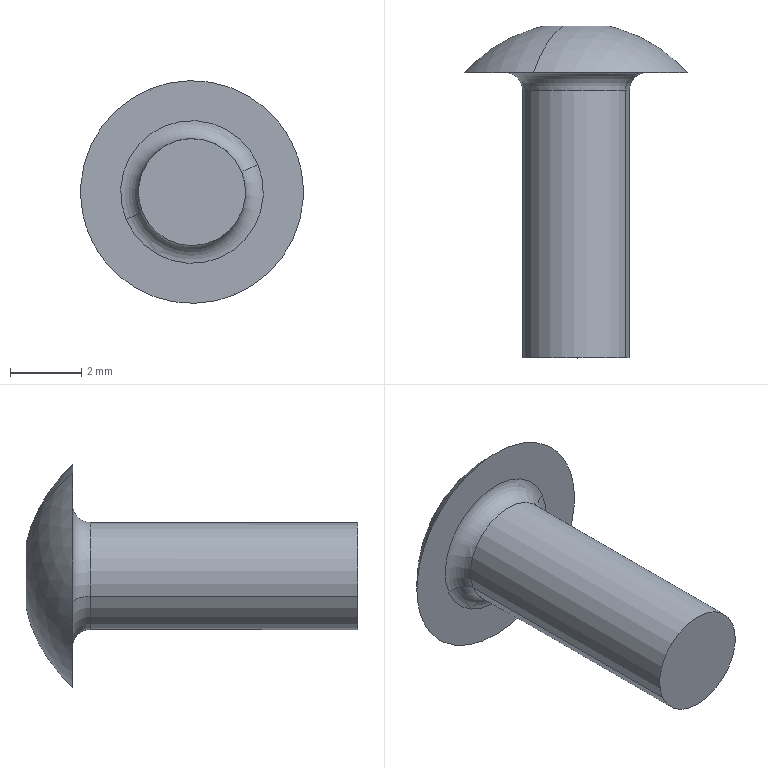Part | SolidWorks | features BaseBody 1 | 1 solid | 9 faces | box 6.24 x 9.303 x 6.24 mm | volume 79.81 mm3 | plane 3 | sphere 2 | torus 2 | cylinder 2 | commonest cylinder face diameters 3 x2
STEP:
#1=CARTESIAN_POINT('',(-240.642,13.167,-31.72));
#2=VERTEX_POINT('',#1);
#3=CARTESIAN_POINT('',(-241.341,14.088,-30.023));
#4=VERTEX_POINT('',#3);
#5=CARTESIAN_POINT('',(-241.684,10.009,-29.193));
#6=DIRECTION('',(0.9245,-0.0001344,0.3811));
#7=DIRECTION('',(0.3811,0.,-0.9245));
#8=AXIS2_PLACEMENT_3D('',#5,#6,#7);
#9=CIRCLE('',#8,4.177);
#10=EDGE_CURVE('',#2,#4,#9,.T.);
#11=ORIENTED_EDGE('',*,*,#10,.F.);
#12=CARTESIAN_POINT('',(-240.495,12.787,-32.076));
#13=VERTEX_POINT('',#12);
#14=CARTESIAN_POINT('',(-241.684,10.009,-29.193));
#15=DIRECTION('',(-0.9245,0.0001344,-0.3811));
#16=DIRECTION('',(-0.3811,0.,0.9245));
#17=AXIS2_PLACEMENT_3D('',#14,#15,#16);
#18=CIRCLE('',#17,4.177);
#19=EDGE_CURVE('',#2,#13,#18,.T.);
#20=ORIENTED_EDGE('',*,*,#19,.T.);
#21=CARTESIAN_POINT('',(-242.873,12.784,-26.307));
#22=VERTEX_POINT('',#21);
#23=CARTESIAN_POINT('',(-241.684,12.786,-29.192));
#24=DIRECTION('',(0.00003827,-1.,-0.0004455));
#25=DIRECTION('',(0.9245,-0.0001344,0.3811));
#26=AXIS2_PLACEMENT_3D('',#23,#24,#25);
#27=CIRCLE('',#26,3.12);
#28=EDGE_CURVE('',#22,#13,#27,.T.);
#29=ORIENTED_EDGE('',*,*,#28,.F.);
#30=CARTESIAN_POINT('',(-242.027,14.087,-28.359));
#31=VERTEX_POINT('',#30);
#32=CARTESIAN_POINT('',(-241.684,10.009,-29.193));
#33=DIRECTION('',(0.9245,-0.0001344,0.3811));
#34=DIRECTION('',(0.3811,0.,-0.9245));
#35=AXIS2_PLACEMENT_3D('',#32,#33,#34);
#36=CIRCLE('',#35,4.177);
#37=EDGE_CURVE('',#31,#22,#36,.T.);
#38=ORIENTED_EDGE('',*,*,#37,.F.);
#39=CARTESIAN_POINT('',(-241.684,14.088,-29.191));
#40=DIRECTION('',(-0.00003827,1.,0.0004455));
#41=DIRECTION('',(0.9245,-0.0001344,0.3811));
#42=AXIS2_PLACEMENT_3D('',#39,#40,#41);
#43=CIRCLE('',#42,0.9);
#44=EDGE_CURVE('',#4,#31,#43,.T.);
#45=ORIENTED_EDGE('',*,*,#44,.F.);
#46=EDGE_LOOP('',(#11,#20,#29,#38,#45));
#47=FACE_OUTER_BOUND('',#46,.T.);
#48=CARTESIAN_POINT('',(-241.684,10.009,-29.193));
#49=DIRECTION('',(-0.9245,0.0001344,-0.3811));
#50=DIRECTION('',(-0.288,0.6545,0.6991));
#51=AXIS2_PLACEMENT_3D('',#48,#49,#50);
#52=SPHERICAL_SURFACE('',#51,4.177);
#53=ADVANCED_FACE('',(#47),#52,.T.);
#54=CARTESIAN_POINT('',(-240.297,12.285,-28.62));
#55=VERTEX_POINT('',#54);
#56=CARTESIAN_POINT('',(-243.071,12.286,-29.763));
#57=VERTEX_POINT('',#56);
#58=CARTESIAN_POINT('',(-241.684,12.286,-29.192));
#59=DIRECTION('',(0.00003827,-1.,-0.0004455));
#60=DIRECTION('',(0.9245,-0.0001344,0.3811));
#61=AXIS2_PLACEMENT_3D('',#58,#59,#60);
#62=CIRCLE('',#61,1.5);
#63=EDGE_CURVE('',#55,#57,#62,.T.);
#64=ORIENTED_EDGE('',*,*,#63,.F.);
#65=CARTESIAN_POINT('',(-239.835,12.785,-28.429));
#66=VERTEX_POINT('',#65);
#67=CARTESIAN_POINT('',(-239.835,12.285,-28.43));
#68=DIRECTION('',(-0.3811,-0.0004264,0.9245));
#69=DIRECTION('',(-0.00003827,1.,0.0004455));
#70=AXIS2_PLACEMENT_3D('',#67,#68,#69);
#71=CIRCLE('',#70,0.5);
#72=EDGE_CURVE('',#66,#55,#71,.T.);
#73=ORIENTED_EDGE('',*,*,#72,.F.);
#74=CARTESIAN_POINT('',(-243.533,12.786,-29.954));
#75=VERTEX_POINT('',#74);
#76=CARTESIAN_POINT('',(-241.684,12.786,-29.192));
#77=DIRECTION('',(0.00003827,-1.,-0.0004455));
#78=DIRECTION('',(0.9245,-0.0001344,0.3811));
#79=AXIS2_PLACEMENT_3D('',#76,#77,#78);
#80=CIRCLE('',#79,2.);
#81=EDGE_CURVE('',#66,#75,#80,.T.);
#82=ORIENTED_EDGE('',*,*,#81,.T.);
#83=CARTESIAN_POINT('',(-243.533,12.286,-29.954));
#84=DIRECTION('',(0.3811,0.0004264,-0.9245));
#85=DIRECTION('',(-0.00003827,1.,0.0004455));
#86=AXIS2_PLACEMENT_3D('',#83,#84,#85);
#87=CIRCLE('',#86,0.5);
#88=EDGE_CURVE('',#75,#57,#87,.T.);
#89=ORIENTED_EDGE('',*,*,#88,.T.);
#90=EDGE_LOOP('',(#64,#73,#82,#89));
#91=FACE_OUTER_BOUND('',#90,.T.);
#92=CARTESIAN_POINT('',(-241.684,12.286,-29.192));
#93=DIRECTION('',(-0.00003827,1.,0.0004455));
#94=DIRECTION('',(-0.9245,0.0001344,-0.3811));
#95=AXIS2_PLACEMENT_3D('',#92,#93,#94);
#96=TOROIDAL_SURFACE('',#95,2.,0.5);
#97=ADVANCED_FACE('',(#91),#96,.F.);
#98=ORIENTED_EDGE('',*,*,#88,.F.);
#99=CARTESIAN_POINT('',(-241.684,12.786,-29.192));
#100=DIRECTION('',(0.00003827,-1.,-0.0004455));
#101=DIRECTION('',(-0.9245,0.0001344,-0.3811));
#102=AXIS2_PLACEMENT_3D('',#99,#100,#101);
#103=CIRCLE('',#102,2.);
#104=EDGE_CURVE('',#75,#66,#103,.T.);
#105=ORIENTED_EDGE('',*,*,#104,.T.);
#106=ORIENTED_EDGE('',*,*,#72,.T.);
#107=CARTESIAN_POINT('',(-241.684,12.286,-29.192));
#108=DIRECTION('',(0.00003827,-1.,-0.0004455));
#109=DIRECTION('',(-0.9245,0.0001344,-0.3811));
#110=AXIS2_PLACEMENT_3D('',#107,#108,#109);
#111=CIRCLE('',#110,1.5);
#112=EDGE_CURVE('',#57,#55,#111,.T.);
#113=ORIENTED_EDGE('',*,*,#112,.F.);
#114=EDGE_LOOP('',(#98,#105,#106,#113));
#115=FACE_OUTER_BOUND('',#114,.T.);
#116=CARTESIAN_POINT('',(-241.684,12.286,-29.192));
#117=DIRECTION('',(-0.00003827,1.,0.0004455));
#118=DIRECTION('',(0.9245,-0.0001344,0.3811));
#119=AXIS2_PLACEMENT_3D('',#116,#117,#118);
#120=TOROIDAL_SURFACE('',#119,2.,0.5);
#121=ADVANCED_FACE('',(#115),#120,.F.);
#122=CARTESIAN_POINT('',(-243.07,4.786,-29.767));
#123=VERTEX_POINT('',#122);
#124=CARTESIAN_POINT('',(-243.071,12.286,-29.763));
#125=DIRECTION('',(0.00003827,-1.,-0.0004455));
#126=VECTOR('',#125,1000.);
#127=LINE('',#124,#126);
#128=EDGE_CURVE('',#57,#123,#127,.T.);
#129=ORIENTED_EDGE('',*,*,#128,.F.);
#130=ORIENTED_EDGE('',*,*,#112,.T.);
#131=CARTESIAN_POINT('',(-240.297,4.785,-28.624));
#132=VERTEX_POINT('',#131);
#133=CARTESIAN_POINT('',(-240.297,12.285,-28.62));
#134=DIRECTION('',(0.00003827,-1.,-0.0004455));
#135=VECTOR('',#134,1000.);
#136=LINE('',#133,#135);
#137=EDGE_CURVE('',#55,#132,#136,.T.);
#138=ORIENTED_EDGE('',*,*,#137,.T.);
#139=CARTESIAN_POINT('',(-241.684,4.786,-29.195));
#140=DIRECTION('',(-0.00003827,1.,0.0004455));
#141=DIRECTION('',(0.9245,-0.0001344,0.3811));
#142=AXIS2_PLACEMENT_3D('',#139,#140,#141);
#143=CIRCLE('',#142,1.5);
#144=EDGE_CURVE('',#132,#123,#143,.T.);
#145=ORIENTED_EDGE('',*,*,#144,.T.);
#146=EDGE_LOOP('',(#129,#130,#138,#145));
#147=FACE_OUTER_BOUND('',#146,.T.);
#148=CARTESIAN_POINT('',(-241.684,24.02,-29.187));
#149=DIRECTION('',(-0.00003827,1.,0.0004455));
#150=DIRECTION('',(0.9245,-0.0001344,0.3811));
#151=AXIS2_PLACEMENT_3D('',#148,#149,#150);
#152=CYLINDRICAL_SURFACE('',#151,1.5);
#153=ADVANCED_FACE('',(#147),#152,.T.);
#154=CARTESIAN_POINT('',(-241.684,4.786,-29.195));
#155=DIRECTION('',(-0.00003827,1.,0.0004455));
#156=DIRECTION('',(-0.9245,0.0001344,-0.3811));
#157=AXIS2_PLACEMENT_3D('',#154,#155,#156);
#158=CIRCLE('',#157,1.5);
#159=EDGE_CURVE('',#123,#132,#158,.T.);
#160=ORIENTED_EDGE('',*,*,#159,.F.);
#161=ORIENTED_EDGE('',*,*,#144,.F.);
#162=EDGE_LOOP('',(#160,#161));
#163=FACE_OUTER_BOUND('',#162,.T.);
#164=CARTESIAN_POINT('',(-242.516,4.786,-29.538));
#165=DIRECTION('',(-0.00003827,1.,0.0004455));
#166=DIRECTION('',(0.9963,0.,0.08559));
#167=AXIS2_PLACEMENT_3D('',#164,#165,#166);
#168=PLANE('',#167);
#169=ADVANCED_FACE('',(#163),#168,.F.);
#170=ORIENTED_EDGE('',*,*,#159,.T.);
#171=ORIENTED_EDGE('',*,*,#137,.F.);
#172=ORIENTED_EDGE('',*,*,#63,.T.);
#173=ORIENTED_EDGE('',*,*,#128,.T.);
#174=EDGE_LOOP('',(#170,#171,#172,#173));
#175=FACE_OUTER_BOUND('',#174,.T.);
#176=CARTESIAN_POINT('',(-241.684,24.02,-29.187));
#177=DIRECTION('',(-0.00003827,1.,0.0004455));
#178=DIRECTION('',(0.9245,-0.0001344,0.3811));
#179=AXIS2_PLACEMENT_3D('',#176,#177,#178);
#180=CYLINDRICAL_SURFACE('',#179,1.5);
#181=ADVANCED_FACE('',(#175),#180,.T.);
#182=ORIENTED_EDGE('',*,*,#104,.F.);
#183=ORIENTED_EDGE('',*,*,#81,.F.);
#184=EDGE_LOOP('',(#182,#183));
#185=FACE_BOUND('',#184,.T.);
#186=ORIENTED_EDGE('',*,*,#28,.T.);
#187=CARTESIAN_POINT('',(-241.684,12.786,-29.192));
#188=DIRECTION('',(0.00003827,-1.,-0.0004455));
#189=DIRECTION('',(0.9245,-0.0001344,0.3811));
#190=AXIS2_PLACEMENT_3D('',#187,#188,#189);
#191=CIRCLE('',#190,3.12);
#192=EDGE_CURVE('',#13,#22,#191,.T.);
#193=ORIENTED_EDGE('',*,*,#192,.T.);
#194=EDGE_LOOP('',(#186,#193));
#195=FACE_OUTER_BOUND('',#194,.T.);
#196=CARTESIAN_POINT('',(-243.071,12.786,-29.763));
#197=DIRECTION('',(-0.00003827,1.,0.0004455));
#198=DIRECTION('',(0.9963,0.,0.08559));
#199=AXIS2_PLACEMENT_3D('',#196,#197,#198);
#200=PLANE('',#199);
#201=ADVANCED_FACE('',(#185,#195),#200,.F.);
#202=ORIENTED_EDGE('',*,*,#19,.F.);
#203=ORIENTED_EDGE('',*,*,#10,.T.);
#204=CARTESIAN_POINT('',(-241.684,14.088,-29.191));
#205=DIRECTION('',(-0.00003827,1.,0.0004455));
#206=DIRECTION('',(0.9245,-0.0001344,0.3811));
#207=AXIS2_PLACEMENT_3D('',#204,#205,#206);
#208=CIRCLE('',#207,0.9);
#209=EDGE_CURVE('',#31,#4,#208,.T.);
#210=ORIENTED_EDGE('',*,*,#209,.F.);
#211=ORIENTED_EDGE('',*,*,#37,.T.);
#212=ORIENTED_EDGE('',*,*,#192,.F.);
#213=EDGE_LOOP('',(#202,#203,#210,#211,#212));
#214=FACE_OUTER_BOUND('',#213,.T.);
#215=CARTESIAN_POINT('',(-241.684,10.009,-29.193));
#216=DIRECTION('',(-0.9245,0.0001344,-0.3811));
#217=DIRECTION('',(-0.288,0.6545,0.6991));
#218=AXIS2_PLACEMENT_3D('',#215,#216,#217);
#219=SPHERICAL_SURFACE('',#218,4.177);
#220=ADVANCED_FACE('',(#214),#219,.T.);
#221=ORIENTED_EDGE('',*,*,#44,.T.);
#222=ORIENTED_EDGE('',*,*,#209,.T.);
#223=EDGE_LOOP('',(#221,#222));
#224=FACE_OUTER_BOUND('',#223,.T.);
#225=CARTESIAN_POINT('',(-241.684,14.088,-29.191));
#226=DIRECTION('',(-0.00003827,1.,0.0004455));
#227=DIRECTION('',(0.9963,0.,0.08559));
#228=AXIS2_PLACEMENT_3D('',#225,#226,#227);
#229=PLANE('',#228);
#230=ADVANCED_FACE('',(#224),#229,.T.);
#231=CLOSED_SHELL('',(#53,#97,#121,#153,#169,#181,#201,#220,#230));
#232=MANIFOLD_SOLID_BREP('',#231);
#233=CARTESIAN_POINT('',(0.,0.,0.));
#234=DIRECTION('',(0.,0.,1.));
#235=DIRECTION('',(1.,0.,0.));
#236=AXIS2_PLACEMENT_3D('',#233,#234,#235);
#237=(LENGTH_UNIT()NAMED_UNIT(*)SI_UNIT(.MILLI.,.METRE.));
#238=UNCERTAINTY_MEASURE_WITH_UNIT(LENGTH_MEASURE(0.00001),#237,'','');
#239=(NAMED_UNIT(*)PLANE_ANGLE_UNIT()SI_UNIT($,.RADIAN.));
#240=(NAMED_UNIT(*)SI_UNIT($,.STERADIAN.)SOLID_ANGLE_UNIT());
#241=(GEOMETRIC_REPRESENTATION_CONTEXT(3)GLOBAL_UNCERTAINTY_ASSIGNED_CONTEXT((#238))GLOBAL_UNIT_ASSIGNED_CONTEXT((#237,#239,#240))REPRESENTATION_CONTEXT('',''));
#242=ADVANCED_BREP_SHAPE_REPRESENTATION('',(#232,#236),#241);